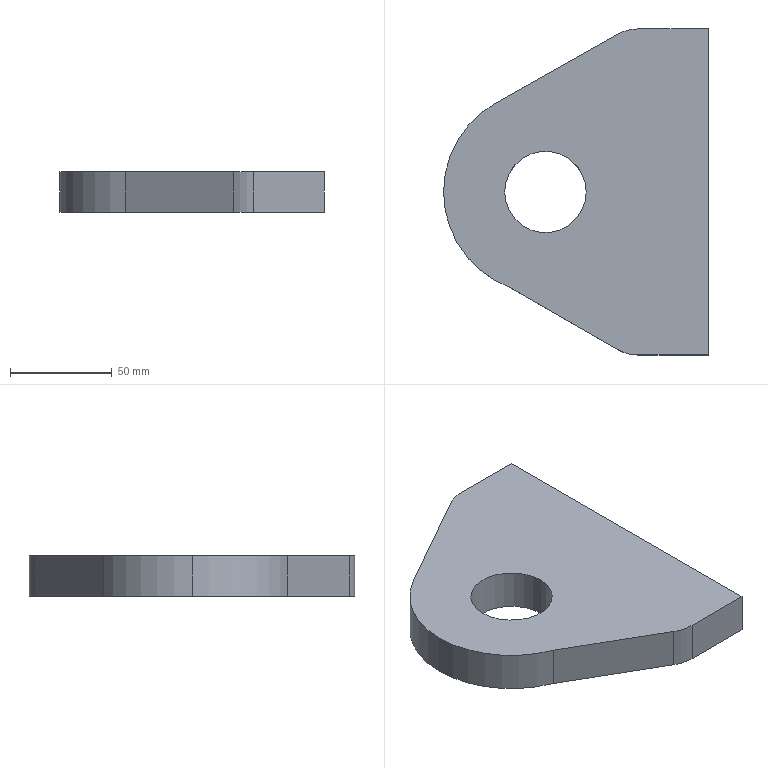Part | SolidWorks | features BaseBody 1 | 1 solid | 13 faces | box 130 x 160 x 20 mm | volume 293365 mm3 | plane 7 | cylinder 6 | commonest cylinder face diameters 40 x4 100 x2
STEP:
#1=CARTESIAN_POINT('',(-20.,0.,10.));
#2=VERTEX_POINT('',#1);
#3=CARTESIAN_POINT('',(20.,0.,10.));
#4=VERTEX_POINT('',#3);
#5=CARTESIAN_POINT('',(0.,0.,10.));
#6=DIRECTION('',(0.,0.,1.));
#7=DIRECTION('',(1.,0.,0.));
#8=AXIS2_PLACEMENT_3D('',#5,#6,#7);
#9=CIRCLE('',#8,20.);
#10=EDGE_CURVE('',#2,#4,#9,.T.);
#11=ORIENTED_EDGE('',*,*,#10,.T.);
#12=CARTESIAN_POINT('',(20.,0.,-10.));
#13=VERTEX_POINT('',#12);
#14=CARTESIAN_POINT('',(20.,0.,10.));
#15=DIRECTION('',(0.,0.,-1.));
#16=VECTOR('',#15,1000.);
#17=LINE('',#14,#16);
#18=EDGE_CURVE('',#4,#13,#17,.T.);
#19=ORIENTED_EDGE('',*,*,#18,.T.);
#20=CARTESIAN_POINT('',(-20.,0.,-10.));
#21=VERTEX_POINT('',#20);
#22=CARTESIAN_POINT('',(0.,0.,-10.));
#23=DIRECTION('',(0.,0.,1.));
#24=DIRECTION('',(1.,0.,0.));
#25=AXIS2_PLACEMENT_3D('',#22,#23,#24);
#26=CIRCLE('',#25,20.);
#27=EDGE_CURVE('',#21,#13,#26,.T.);
#28=ORIENTED_EDGE('',*,*,#27,.F.);
#29=CARTESIAN_POINT('',(-20.,0.,10.));
#30=DIRECTION('',(0.,0.,-1.));
#31=VECTOR('',#30,1000.);
#32=LINE('',#29,#31);
#33=EDGE_CURVE('',#2,#21,#32,.T.);
#34=ORIENTED_EDGE('',*,*,#33,.F.);
#35=EDGE_LOOP('',(#11,#19,#28,#34));
#36=FACE_OUTER_BOUND('',#35,.T.);
#37=CARTESIAN_POINT('',(0.,0.,10.));
#38=DIRECTION('',(0.,0.,-1.));
#39=DIRECTION('',(-1.,0.,0.));
#40=AXIS2_PLACEMENT_3D('',#37,#38,#39);
#41=CYLINDRICAL_SURFACE('',#40,20.);
#42=ADVANCED_FACE('',(#36),#41,.F.);
#43=CARTESIAN_POINT('',(-50.,0.,10.));
#44=VERTEX_POINT('',#43);
#45=CARTESIAN_POINT('',(-17.72,-46.755,10.));
#46=VERTEX_POINT('',#45);
#47=CARTESIAN_POINT('',(0.,0.,10.));
#48=DIRECTION('',(0.,0.,1.));
#49=DIRECTION('',(1.,0.,0.));
#50=AXIS2_PLACEMENT_3D('',#47,#48,#49);
#51=CIRCLE('',#50,50.);
#52=EDGE_CURVE('',#44,#46,#51,.T.);
#53=ORIENTED_EDGE('',*,*,#52,.F.);
#54=CARTESIAN_POINT('',(-50.,0.,-10.));
#55=VERTEX_POINT('',#54);
#56=CARTESIAN_POINT('',(-50.,0.,10.));
#57=DIRECTION('',(0.,0.,-1.));
#58=VECTOR('',#57,1000.);
#59=LINE('',#56,#58);
#60=EDGE_CURVE('',#44,#55,#59,.T.);
#61=ORIENTED_EDGE('',*,*,#60,.T.);
#62=CARTESIAN_POINT('',(-17.72,-46.755,-10.));
#63=VERTEX_POINT('',#62);
#64=CARTESIAN_POINT('',(0.,0.,-10.));
#65=DIRECTION('',(0.,0.,1.));
#66=DIRECTION('',(1.,0.,0.));
#67=AXIS2_PLACEMENT_3D('',#64,#65,#66);
#68=CIRCLE('',#67,50.);
#69=EDGE_CURVE('',#55,#63,#68,.T.);
#70=ORIENTED_EDGE('',*,*,#69,.T.);
#71=CARTESIAN_POINT('',(-17.72,-46.755,10.));
#72=DIRECTION('',(0.,0.,-1.));
#73=VECTOR('',#72,1000.);
#74=LINE('',#71,#73);
#75=EDGE_CURVE('',#46,#63,#74,.T.);
#76=ORIENTED_EDGE('',*,*,#75,.F.);
#77=EDGE_LOOP('',(#53,#61,#70,#76));
#78=FACE_OUTER_BOUND('',#77,.T.);
#79=CARTESIAN_POINT('',(0.,0.,10.));
#80=DIRECTION('',(0.,0.,-1.));
#81=DIRECTION('',(-1.,0.,0.));
#82=AXIS2_PLACEMENT_3D('',#79,#80,#81);
#83=CYLINDRICAL_SURFACE('',#82,50.);
#84=ADVANCED_FACE('',(#78),#83,.T.);
#85=CARTESIAN_POINT('',(45.256,80.,10.));
#86=VERTEX_POINT('',#85);
#87=CARTESIAN_POINT('',(35.423,77.416,10.));
#88=VERTEX_POINT('',#87);
#89=CARTESIAN_POINT('',(45.256,60.,10.));
#90=DIRECTION('',(0.,0.,1.));
#91=DIRECTION('',(1.,0.,0.));
#92=AXIS2_PLACEMENT_3D('',#89,#90,#91);
#93=CIRCLE('',#92,20.);
#94=EDGE_CURVE('',#86,#88,#93,.T.);
#95=ORIENTED_EDGE('',*,*,#94,.T.);
#96=CARTESIAN_POINT('',(-24.581,43.54,10.));
#97=VERTEX_POINT('',#96);
#98=CARTESIAN_POINT('',(35.423,77.416,10.));
#99=DIRECTION('',(-0.8708,-0.4916,0.));
#100=VECTOR('',#99,1000.);
#101=LINE('',#98,#100);
#102=EDGE_CURVE('',#88,#97,#101,.T.);
#103=ORIENTED_EDGE('',*,*,#102,.T.);
#104=CARTESIAN_POINT('',(0.,0.,10.));
#105=DIRECTION('',(0.,0.,1.));
#106=DIRECTION('',(1.,0.,0.));
#107=AXIS2_PLACEMENT_3D('',#104,#105,#106);
#108=CIRCLE('',#107,50.);
#109=EDGE_CURVE('',#97,#44,#108,.T.);
#110=ORIENTED_EDGE('',*,*,#109,.T.);
#111=ORIENTED_EDGE('',*,*,#52,.T.);
#112=CARTESIAN_POINT('',(35.366,-77.331,10.));
#113=VERTEX_POINT('',#112);
#114=CARTESIAN_POINT('',(35.366,-77.331,10.));
#115=DIRECTION('',(0.8665,-0.4991,0.));
#116=VECTOR('',#115,1000.);
#117=LINE('',#114,#116);
#118=EDGE_CURVE('',#46,#113,#117,.T.);
#119=ORIENTED_EDGE('',*,*,#118,.T.);
#120=CARTESIAN_POINT('',(45.348,-80.,10.));
#121=VERTEX_POINT('',#120);
#122=CARTESIAN_POINT('',(45.348,-60.,10.));
#123=DIRECTION('',(0.,0.,1.));
#124=DIRECTION('',(1.,0.,0.));
#125=AXIS2_PLACEMENT_3D('',#122,#123,#124);
#126=CIRCLE('',#125,20.);
#127=EDGE_CURVE('',#113,#121,#126,.T.);
#128=ORIENTED_EDGE('',*,*,#127,.T.);
#129=CARTESIAN_POINT('',(80.,-80.,10.));
#130=VERTEX_POINT('',#129);
#131=CARTESIAN_POINT('',(80.,-80.,10.));
#132=DIRECTION('',(1.,0.,0.));
#133=VECTOR('',#132,1000.);
#134=LINE('',#131,#133);
#135=EDGE_CURVE('',#121,#130,#134,.T.);
#136=ORIENTED_EDGE('',*,*,#135,.T.);
#137=CARTESIAN_POINT('',(80.,80.,10.));
#138=VERTEX_POINT('',#137);
#139=CARTESIAN_POINT('',(80.,80.,10.));
#140=DIRECTION('',(0.,1.,0.));
#141=VECTOR('',#140,1000.);
#142=LINE('',#139,#141);
#143=EDGE_CURVE('',#130,#138,#142,.T.);
#144=ORIENTED_EDGE('',*,*,#143,.T.);
#145=CARTESIAN_POINT('',(80.,80.,10.));
#146=DIRECTION('',(-1.,0.,0.));
#147=VECTOR('',#146,1000.);
#148=LINE('',#145,#147);
#149=EDGE_CURVE('',#138,#86,#148,.T.);
#150=ORIENTED_EDGE('',*,*,#149,.T.);
#151=EDGE_LOOP('',(#95,#103,#110,#111,#119,#128,#136,#144,#150));
#152=FACE_OUTER_BOUND('',#151,.T.);
#153=ORIENTED_EDGE('',*,*,#10,.F.);
#154=CARTESIAN_POINT('',(0.,0.,10.));
#155=DIRECTION('',(0.,0.,1.));
#156=DIRECTION('',(1.,0.,0.));
#157=AXIS2_PLACEMENT_3D('',#154,#155,#156);
#158=CIRCLE('',#157,20.);
#159=EDGE_CURVE('',#4,#2,#158,.T.);
#160=ORIENTED_EDGE('',*,*,#159,.F.);
#161=EDGE_LOOP('',(#153,#160));
#162=FACE_BOUND('',#161,.T.);
#163=CARTESIAN_POINT('',(45.256,60.,10.));
#164=DIRECTION('',(0.,0.,1.));
#165=DIRECTION('',(1.,0.,0.));
#166=AXIS2_PLACEMENT_3D('',#163,#164,#165);
#167=PLANE('',#166);
#168=ADVANCED_FACE('',(#152,#162),#167,.T.);
#169=CARTESIAN_POINT('',(45.256,80.,-10.));
#170=VERTEX_POINT('',#169);
#171=CARTESIAN_POINT('',(35.423,77.416,-10.));
#172=VERTEX_POINT('',#171);
#173=CARTESIAN_POINT('',(45.256,60.,-10.));
#174=DIRECTION('',(0.,0.,1.));
#175=DIRECTION('',(1.,0.,0.));
#176=AXIS2_PLACEMENT_3D('',#173,#174,#175);
#177=CIRCLE('',#176,20.);
#178=EDGE_CURVE('',#170,#172,#177,.T.);
#179=ORIENTED_EDGE('',*,*,#178,.F.);
#180=CARTESIAN_POINT('',(80.,80.,-10.));
#181=VERTEX_POINT('',#180);
#182=CARTESIAN_POINT('',(80.,80.,-10.));
#183=DIRECTION('',(-1.,0.,0.));
#184=VECTOR('',#183,1000.);
#185=LINE('',#182,#184);
#186=EDGE_CURVE('',#181,#170,#185,.T.);
#187=ORIENTED_EDGE('',*,*,#186,.F.);
#188=CARTESIAN_POINT('',(80.,-80.,-10.));
#189=VERTEX_POINT('',#188);
#190=CARTESIAN_POINT('',(80.,80.,-10.));
#191=DIRECTION('',(0.,1.,0.));
#192=VECTOR('',#191,1000.);
#193=LINE('',#190,#192);
#194=EDGE_CURVE('',#189,#181,#193,.T.);
#195=ORIENTED_EDGE('',*,*,#194,.F.);
#196=CARTESIAN_POINT('',(45.348,-80.,-10.));
#197=VERTEX_POINT('',#196);
#198=CARTESIAN_POINT('',(80.,-80.,-10.));
#199=DIRECTION('',(1.,0.,0.));
#200=VECTOR('',#199,1000.);
#201=LINE('',#198,#200);
#202=EDGE_CURVE('',#197,#189,#201,.T.);
#203=ORIENTED_EDGE('',*,*,#202,.F.);
#204=CARTESIAN_POINT('',(35.366,-77.331,-10.));
#205=VERTEX_POINT('',#204);
#206=CARTESIAN_POINT('',(45.348,-60.,-10.));
#207=DIRECTION('',(0.,0.,1.));
#208=DIRECTION('',(1.,0.,0.));
#209=AXIS2_PLACEMENT_3D('',#206,#207,#208);
#210=CIRCLE('',#209,20.);
#211=EDGE_CURVE('',#205,#197,#210,.T.);
#212=ORIENTED_EDGE('',*,*,#211,.F.);
#213=CARTESIAN_POINT('',(35.366,-77.331,-10.));
#214=DIRECTION('',(0.8665,-0.4991,0.));
#215=VECTOR('',#214,1000.);
#216=LINE('',#213,#215);
#217=EDGE_CURVE('',#63,#205,#216,.T.);
#218=ORIENTED_EDGE('',*,*,#217,.F.);
#219=ORIENTED_EDGE('',*,*,#69,.F.);
#220=CARTESIAN_POINT('',(-24.581,43.54,-10.));
#221=VERTEX_POINT('',#220);
#222=CARTESIAN_POINT('',(0.,0.,-10.));
#223=DIRECTION('',(0.,0.,1.));
#224=DIRECTION('',(1.,0.,0.));
#225=AXIS2_PLACEMENT_3D('',#222,#223,#224);
#226=CIRCLE('',#225,50.);
#227=EDGE_CURVE('',#221,#55,#226,.T.);
#228=ORIENTED_EDGE('',*,*,#227,.F.);
#229=CARTESIAN_POINT('',(35.423,77.416,-10.));
#230=DIRECTION('',(-0.8708,-0.4916,0.));
#231=VECTOR('',#230,1000.);
#232=LINE('',#229,#231);
#233=EDGE_CURVE('',#172,#221,#232,.T.);
#234=ORIENTED_EDGE('',*,*,#233,.F.);
#235=EDGE_LOOP('',(#179,#187,#195,#203,#212,#218,#219,#228,#234));
#236=FACE_OUTER_BOUND('',#235,.T.);
#237=ORIENTED_EDGE('',*,*,#27,.T.);
#238=CARTESIAN_POINT('',(0.,0.,-10.));
#239=DIRECTION('',(0.,0.,1.));
#240=DIRECTION('',(1.,0.,0.));
#241=AXIS2_PLACEMENT_3D('',#238,#239,#240);
#242=CIRCLE('',#241,20.);
#243=EDGE_CURVE('',#13,#21,#242,.T.);
#244=ORIENTED_EDGE('',*,*,#243,.T.);
#245=EDGE_LOOP('',(#237,#244));
#246=FACE_BOUND('',#245,.T.);
#247=CARTESIAN_POINT('',(45.256,60.,-10.));
#248=DIRECTION('',(0.,0.,1.));
#249=DIRECTION('',(1.,0.,0.));
#250=AXIS2_PLACEMENT_3D('',#247,#248,#249);
#251=PLANE('',#250);
#252=ADVANCED_FACE('',(#236,#246),#251,.F.);
#253=ORIENTED_EDGE('',*,*,#178,.T.);
#254=CARTESIAN_POINT('',(35.423,77.416,10.));
#255=DIRECTION('',(0.,0.,-1.));
#256=VECTOR('',#255,1000.);
#257=LINE('',#254,#256);
#258=EDGE_CURVE('',#88,#172,#257,.T.);
#259=ORIENTED_EDGE('',*,*,#258,.F.);
#260=ORIENTED_EDGE('',*,*,#94,.F.);
#261=CARTESIAN_POINT('',(45.256,80.,10.));
#262=DIRECTION('',(0.,0.,-1.));
#263=VECTOR('',#262,1000.);
#264=LINE('',#261,#263);
#265=EDGE_CURVE('',#86,#170,#264,.T.);
#266=ORIENTED_EDGE('',*,*,#265,.T.);
#267=EDGE_LOOP('',(#253,#259,#260,#266));
#268=FACE_OUTER_BOUND('',#267,.T.);
#269=CARTESIAN_POINT('',(45.256,60.,10.));
#270=DIRECTION('',(0.,0.,-1.));
#271=DIRECTION('',(-1.,0.,0.));
#272=AXIS2_PLACEMENT_3D('',#269,#270,#271);
#273=CYLINDRICAL_SURFACE('',#272,20.);
#274=ADVANCED_FACE('',(#268),#273,.T.);
#275=ORIENTED_EDGE('',*,*,#233,.T.);
#276=CARTESIAN_POINT('',(-24.581,43.54,10.));
#277=DIRECTION('',(0.,0.,-1.));
#278=VECTOR('',#277,1000.);
#279=LINE('',#276,#278);
#280=EDGE_CURVE('',#97,#221,#279,.T.);
#281=ORIENTED_EDGE('',*,*,#280,.F.);
#282=ORIENTED_EDGE('',*,*,#102,.F.);
#283=ORIENTED_EDGE('',*,*,#258,.T.);
#284=EDGE_LOOP('',(#275,#281,#282,#283));
#285=FACE_OUTER_BOUND('',#284,.T.);
#286=CARTESIAN_POINT('',(35.423,77.416,10.));
#287=DIRECTION('',(0.4916,-0.8708,0.));
#288=DIRECTION('',(0.8708,0.4916,0.));
#289=AXIS2_PLACEMENT_3D('',#286,#287,#288);
#290=PLANE('',#289);
#291=ADVANCED_FACE('',(#285),#290,.F.);
#292=ORIENTED_EDGE('',*,*,#60,.F.);
#293=ORIENTED_EDGE('',*,*,#109,.F.);
#294=ORIENTED_EDGE('',*,*,#280,.T.);
#295=ORIENTED_EDGE('',*,*,#227,.T.);
#296=EDGE_LOOP('',(#292,#293,#294,#295));
#297=FACE_OUTER_BOUND('',#296,.T.);
#298=CARTESIAN_POINT('',(0.,0.,10.));
#299=DIRECTION('',(0.,0.,-1.));
#300=DIRECTION('',(-1.,0.,0.));
#301=AXIS2_PLACEMENT_3D('',#298,#299,#300);
#302=CYLINDRICAL_SURFACE('',#301,50.);
#303=ADVANCED_FACE('',(#297),#302,.T.);
#304=ORIENTED_EDGE('',*,*,#217,.T.);
#305=CARTESIAN_POINT('',(35.366,-77.331,10.));
#306=DIRECTION('',(0.,0.,-1.));
#307=VECTOR('',#306,1000.);
#308=LINE('',#305,#307);
#309=EDGE_CURVE('',#113,#205,#308,.T.);
#310=ORIENTED_EDGE('',*,*,#309,.F.);
#311=ORIENTED_EDGE('',*,*,#118,.F.);
#312=ORIENTED_EDGE('',*,*,#75,.T.);
#313=EDGE_LOOP('',(#304,#310,#311,#312));
#314=FACE_OUTER_BOUND('',#313,.T.);
#315=CARTESIAN_POINT('',(35.366,-77.331,10.));
#316=DIRECTION('',(0.4991,0.8665,0.));
#317=DIRECTION('',(-0.8665,0.4991,0.));
#318=AXIS2_PLACEMENT_3D('',#315,#316,#317);
#319=PLANE('',#318);
#320=ADVANCED_FACE('',(#314),#319,.F.);
#321=ORIENTED_EDGE('',*,*,#211,.T.);
#322=CARTESIAN_POINT('',(45.348,-80.,10.));
#323=DIRECTION('',(0.,0.,-1.));
#324=VECTOR('',#323,1000.);
#325=LINE('',#322,#324);
#326=EDGE_CURVE('',#121,#197,#325,.T.);
#327=ORIENTED_EDGE('',*,*,#326,.F.);
#328=ORIENTED_EDGE('',*,*,#127,.F.);
#329=ORIENTED_EDGE('',*,*,#309,.T.);
#330=EDGE_LOOP('',(#321,#327,#328,#329));
#331=FACE_OUTER_BOUND('',#330,.T.);
#332=CARTESIAN_POINT('',(45.348,-60.,10.));
#333=DIRECTION('',(0.,0.,-1.));
#334=DIRECTION('',(-1.,0.,0.));
#335=AXIS2_PLACEMENT_3D('',#332,#333,#334);
#336=CYLINDRICAL_SURFACE('',#335,20.);
#337=ADVANCED_FACE('',(#331),#336,.T.);
#338=ORIENTED_EDGE('',*,*,#202,.T.);
#339=CARTESIAN_POINT('',(80.,-80.,10.));
#340=DIRECTION('',(0.,0.,-1.));
#341=VECTOR('',#340,1000.);
#342=LINE('',#339,#341);
#343=EDGE_CURVE('',#130,#189,#342,.T.);
#344=ORIENTED_EDGE('',*,*,#343,.F.);
#345=ORIENTED_EDGE('',*,*,#135,.F.);
#346=ORIENTED_EDGE('',*,*,#326,.T.);
#347=EDGE_LOOP('',(#338,#344,#345,#346));
#348=FACE_OUTER_BOUND('',#347,.T.);
#349=CARTESIAN_POINT('',(80.,-80.,10.));
#350=DIRECTION('',(0.,1.,0.));
#351=DIRECTION('',(0.,0.,1.));
#352=AXIS2_PLACEMENT_3D('',#349,#350,#351);
#353=PLANE('',#352);
#354=ADVANCED_FACE('',(#348),#353,.F.);
#355=ORIENTED_EDGE('',*,*,#194,.T.);
#356=CARTESIAN_POINT('',(80.,80.,10.));
#357=DIRECTION('',(0.,0.,-1.));
#358=VECTOR('',#357,1000.);
#359=LINE('',#356,#358);
#360=EDGE_CURVE('',#138,#181,#359,.T.);
#361=ORIENTED_EDGE('',*,*,#360,.F.);
#362=ORIENTED_EDGE('',*,*,#143,.F.);
#363=ORIENTED_EDGE('',*,*,#343,.T.);
#364=EDGE_LOOP('',(#355,#361,#362,#363));
#365=FACE_OUTER_BOUND('',#364,.T.);
#366=CARTESIAN_POINT('',(80.,80.,10.));
#367=DIRECTION('',(-1.,0.,0.));
#368=DIRECTION('',(0.,-1.,0.));
#369=AXIS2_PLACEMENT_3D('',#366,#367,#368);
#370=PLANE('',#369);
#371=ADVANCED_FACE('',(#365),#370,.F.);
#372=ORIENTED_EDGE('',*,*,#186,.T.);
#373=ORIENTED_EDGE('',*,*,#265,.F.);
#374=ORIENTED_EDGE('',*,*,#149,.F.);
#375=ORIENTED_EDGE('',*,*,#360,.T.);
#376=EDGE_LOOP('',(#372,#373,#374,#375));
#377=FACE_OUTER_BOUND('',#376,.T.);
#378=CARTESIAN_POINT('',(80.,80.,10.));
#379=DIRECTION('',(0.,-1.,0.));
#380=DIRECTION('',(1.,0.,0.));
#381=AXIS2_PLACEMENT_3D('',#378,#379,#380);
#382=PLANE('',#381);
#383=ADVANCED_FACE('',(#377),#382,.F.);
#384=ORIENTED_EDGE('',*,*,#18,.F.);
#385=ORIENTED_EDGE('',*,*,#159,.T.);
#386=ORIENTED_EDGE('',*,*,#33,.T.);
#387=ORIENTED_EDGE('',*,*,#243,.F.);
#388=EDGE_LOOP('',(#384,#385,#386,#387));
#389=FACE_OUTER_BOUND('',#388,.T.);
#390=CARTESIAN_POINT('',(0.,0.,10.));
#391=DIRECTION('',(0.,0.,-1.));
#392=DIRECTION('',(-1.,0.,0.));
#393=AXIS2_PLACEMENT_3D('',#390,#391,#392);
#394=CYLINDRICAL_SURFACE('',#393,20.);
#395=ADVANCED_FACE('',(#389),#394,.F.);
#396=CLOSED_SHELL('',(#42,#84,#168,#252,#274,#291,#303,#320,#337,#354,#371,#383,#395));
#397=MANIFOLD_SOLID_BREP('',#396);
#398=CARTESIAN_POINT('',(0.,0.,0.));
#399=DIRECTION('',(0.,0.,1.));
#400=DIRECTION('',(1.,0.,0.));
#401=AXIS2_PLACEMENT_3D('',#398,#399,#400);
#402=(LENGTH_UNIT()NAMED_UNIT(*)SI_UNIT(.MILLI.,.METRE.));
#403=UNCERTAINTY_MEASURE_WITH_UNIT(LENGTH_MEASURE(0.00001),#402,'','');
#404=(NAMED_UNIT(*)PLANE_ANGLE_UNIT()SI_UNIT($,.RADIAN.));
#405=(NAMED_UNIT(*)SI_UNIT($,.STERADIAN.)SOLID_ANGLE_UNIT());
#406=(GEOMETRIC_REPRESENTATION_CONTEXT(3)GLOBAL_UNCERTAINTY_ASSIGNED_CONTEXT((#403))GLOBAL_UNIT_ASSIGNED_CONTEXT((#402,#404,#405))REPRESENTATION_CONTEXT('',''));
#407=ADVANCED_BREP_SHAPE_REPRESENTATION('',(#397,#401),#406);